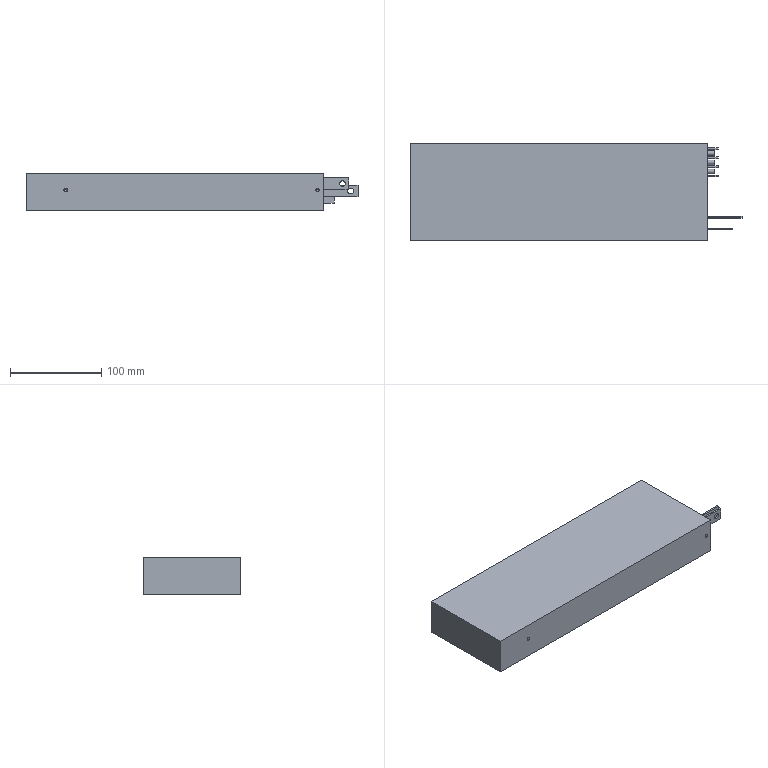Part | STEP file | COMPOUND | 4 solids | 69 faces | box 363.8 x 107 x 41 mm | volume 1432156 mm3 | plane 42 | cone 14 | cylinder 13 | commonest cylinder face diameters 3.3 x4 2.5 x3 5 x3 6.5 x3